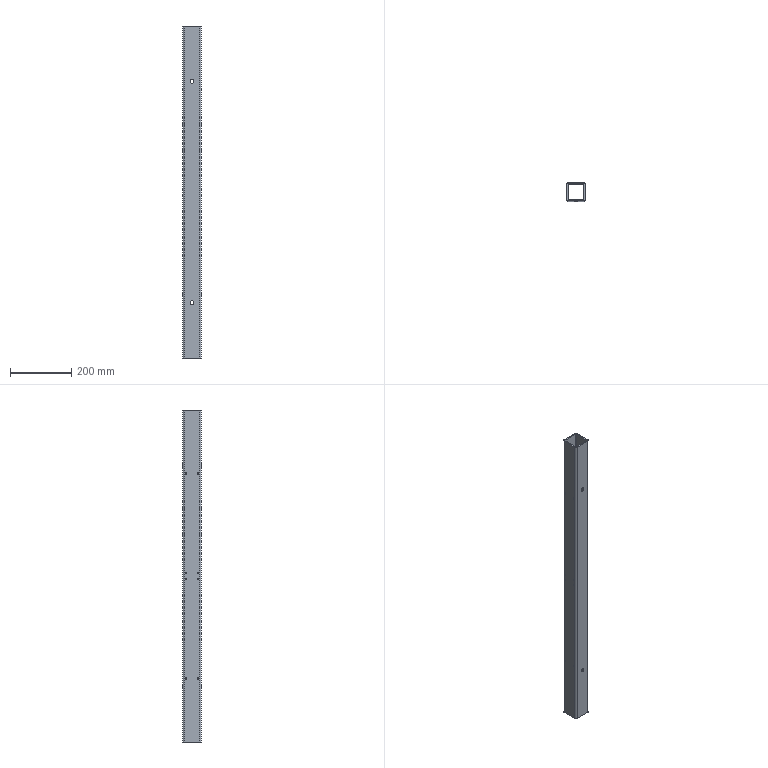Part | STEP file | square steel tube E60x60x4x1080 | 1 solid | 58 faces | box 60 x 60 x 1080 mm | volume 942050 mm3 | cylinder 48 | plane 10 | commonest cylinder face diameters 5 x32 13 x8 2 x4 10 x4